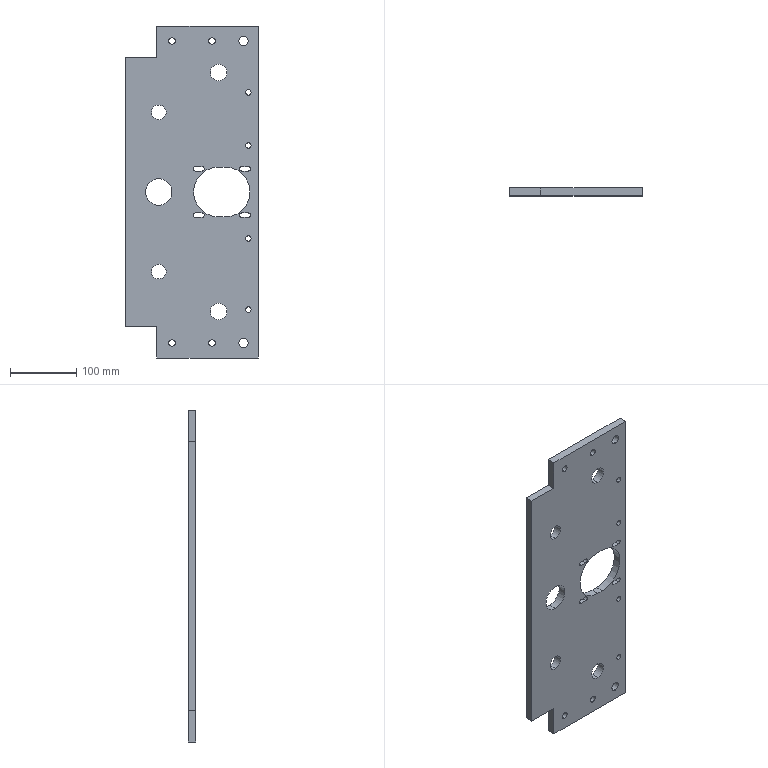Part | SolidWorks | features ICE 7, HoleWzd 3, Fillet 2, Extrusion 1 | 1 solid | 60 faces | box 200 x 12 x 500 mm | volume 1034176 mm3 | cylinder 40 | plane 20 | commonest cylinder face diameters 6.6 x8 8.2 x8 10 x8 14 x4 22 x4 25 x4